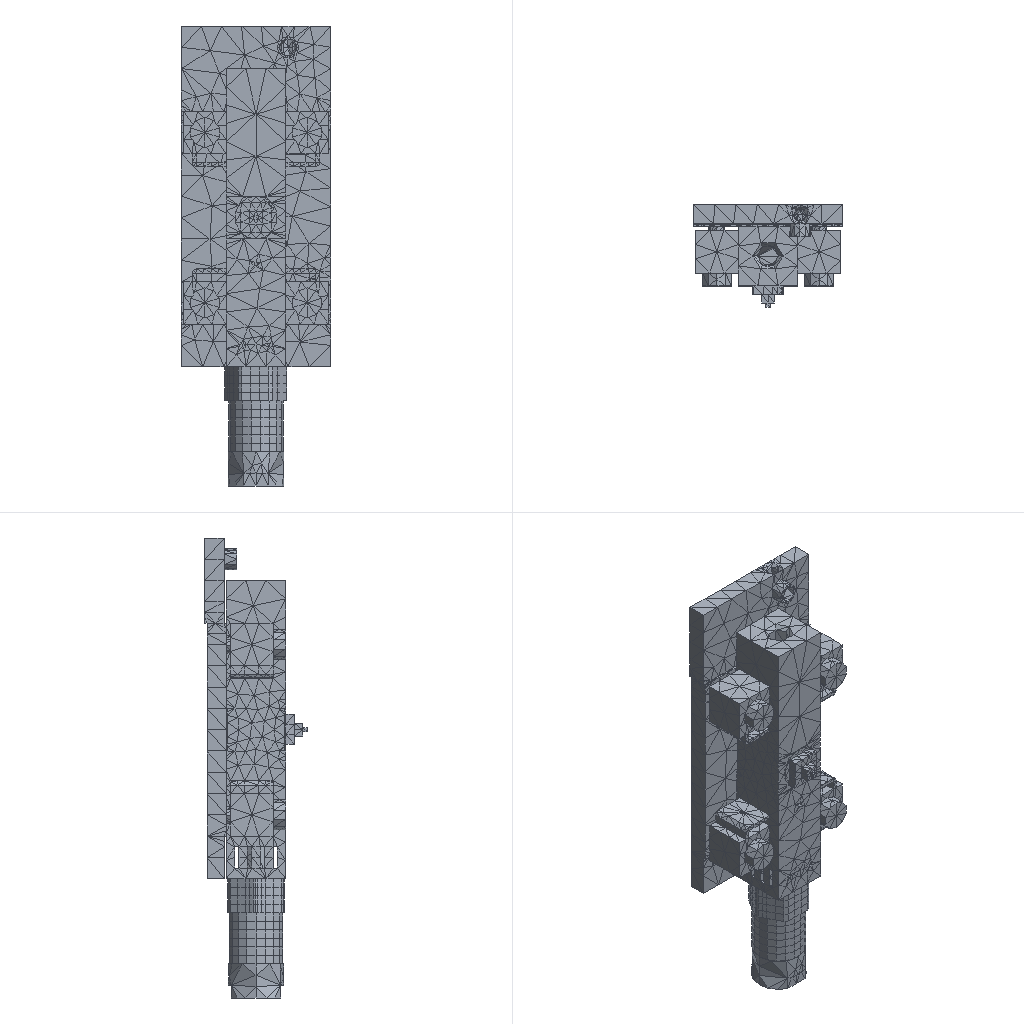Simulation study | ansys workbench
Ansys APDL input file, long lists of numbers shortened:
/batch
/config,noeldb,1     ! force off writing results to database
*get,_wallstrt,active,,time,wall
! ANSYS input file written by Workbench version 2022 R1
! File used for geometry attach: F:\ansys（分析文件汇总)\含底座模态分析\新建文件夹(4)\新建文件夹\完整版.STEP
/title,11111--____ (C5)
! ****** Begin Custom Load Command Snippet ******
/COM, ACT Extensions:
/COM,     LSDYNA, 2021.1
/COM,
! ****** End   Custom Load Command Snippet ******
*DIM,_wb_ProjectScratch_dir,string,248
_wb_ProjectScratch_dir(1) = 'F:\ansys（分析文件汇总)\含底座模态分析\_ProjectScratch\ScrD0BA\'
*DIM,_wb_SolverFiles_dir,string,248
_wb_SolverFiles_dir(1) = 'F:\ansys（分析文件汇总)\含底座模态分析\11111_files\dp0\SYS-1\MECH\'
*DIM,_wb_userfiles_dir,string,248
_wb_userfiles_dir(1) = 'F:\ansys（分析文件汇总)\含底座模态分析\11111_files\user_files\'
/com,--- Data in consistent NMM units. See Solving Units in the help system for more information.
/units,MPA
/nopr
/wb,file,start              !  signify a WB generated input file
/prep7
! Turn off shape checking because checks already performed inside WB mesher.
! See help system for more information.
SHPP,OFF,,NOWARN
/nolist
etcon,set             ! allow ANSYS to choose best KEYOP's for 180x elements, resets any applicable keyopt to MAPDL defaults
/com,*********** Nodes for the whole assembly ***********
nblock,3,,23060
(1i9,3e20.9e3)
        1    -7.593879241E+01     6.122424365E-01     1.555868903E+01
! (20963 more lines like these left out)
-1
/wb,elem,start            !  set before creation of elements
/com,*********** Elements for Body 1 "__|__-__6" ***********
et,1,187
eblock,19,solid,,4865
(19i9)
        1        1        1        1        0        0        0        0       10        0     2024     8034     8303     8491     8312    14700    15906    14703    14701
! (9729 more lines like these left out)
-1
/com,*********** Elements for Body 2 "___|__-__1" ***********
et,2,186
keyo,2,2,1          ! set full integration on SOLID186
eblock,19,solid,,35
(19i9)
        2        2        2        2        0        0        0        0       20        0      840     2544     2556     2561     2557     2579     2567     2562     2566
! (69 more lines like these left out)
-1
/com,*********** Elements for Body 3 "___|__-__1[2]" ***********
et,3,186
keyo,3,2,1          ! set full integration on SOLID186
eblock,19,solid,,35
(19i9)
        3        3        3        3        0        0        0        0       20        0      770     1924     1936     1941     1937     1959     1947     1942     1946
! (69 more lines like these left out)
-1
/com,*********** Elements for Body 4 "___|__-__1[3]" ***********
et,4,186
keyo,4,2,1          ! set full integration on SOLID186
eblock,19,solid,,35
(19i9)
        4        4        4        4        0        0        0        0       20        0      910     3164     3176     3181     3177     3199     3187     3182     3186
! (69 more lines like these left out)
-1
/com,*********** Elements for Body 5 "___|__-__1[4]" ***********
et,5,186
keyo,5,2,1          ! set full integration on SOLID186
eblock,19,solid,,35
(19i9)
        5        5        5        5        0        0        0        0       20        0      805     2234     2246     2251     2247     2269     2257     2252     2256
! (69 more lines like these left out)
-1
! (11 more sections like these left out)
/wb,elem,end               !  done creating elements
/com,*********** Send User Defined Coordinate System(s) ***********
csys,0
toffst,273.15,  ! Temperature offset from absolute zero
/com,*********** Set Reference Temperature ***********
tref,22.
/wb,mat,start              !  starting to send materials
/com,*********** Send Materials ***********
Temperature = 'TEMP' ! Temperature
TB,BISO,1,5,
TBTEMP,100
TBDATA,1,225,2091
TBTEMP,300
TBDATA,1,168,1577
TBTEMP,816
TBDATA,1,115,708
TBTEMP,1040
TBDATA,1,31,405
TBTEMP,1150
TBDATA,1,15,265
MPTEMP,,,,,,,,
MPTEMP,1,20
MPTEMP,2,100
MPTEMP,3,200
MPTEMP,4,300
MPTEMP,5,400
MPTEMP,6,500
MPTEMP,7,600
MPTEMP,8,700
MPTEMP,9,800
MPTEMP,10,900
MPTEMP,11,1000
MPTEMP,12,1100
MPTEMP,13,1200
MPDATA,EX,1, ,195000,191000,186000,180000,173000,164000,
MPDATA,EX,1, ,155000,144000,131000,117000,100000,81000,
MPDATA,EX,1, ,51000,	! tonne s^-2 mm^-1
MPTEMP,,,,,,,,
MPTEMP,,,,,,,,
MPTEMP,1,20
MPTEMP,2,100
MPTEMP,3,200
MPTEMP,4,300
MPTEMP,5,400
MPTEMP,6,500
MPTEMP,7,600
MPTEMP,8,700
MPTEMP,9,800
MPTEMP,10,900
MPTEMP,11,1000
MPTEMP,12,1100
MPTEMP,13,1200
MPDATA,NUXY,1, ,0.25,0.26,0.275,0.315,0.33,0.3,
MPDATA,NUXY,1, ,0.32,0.31,0.24,0.24,0.24,0.24,
MPDATA,NUXY,1, ,0.24,
MPTEMP,,,,,,,,
MPTEMP,,,,,,,,
MPTEMP,1,26.85
MPTEMP,2,126.85
MPTEMP,3,226.85
MPTEMP,4,326.85
MPTEMP,5,426.85
MPTEMP,6,526.85
MPTEMP,7,626.85
MPTEMP,8,726.85
MPTEMP,9,826.85
MPTEMP,10,926.85
MPTEMP,11,1026.85
MPTEMP,12,1126.85
MPTEMP,13,1226.85
MPTEMP,14,1326.85
MPTEMP,15,1426.85
MPTEMP,16,1526.85
MPTEMP,17,1626.85
MPTEMP,18,1726.85
MPTEMP,19,1826.85
MPTEMP,20,1926.85
MPTEMP,21,2026.85
MPTEMP,22,2126.85
MPTEMP,23,2226.85
MPTEMP,24,2326.85
MPTEMP,25,2426.85
MPTEMP,26,2526.85
MPTEMP,27,2626.85
MPTEMP,28,2726.85
MPDATA,DENS,1, ,7.954e-09,7.91e-09,7.864e-09,7.818e-09,7.771e-09,7.723e-09,
MPDATA,DENS,1, ,7.674e-09,7.624e-09,7.574e-09,7.523e-09,7.471e-09,7.419e-09,
! (1352 more lines like these left out)
/wb,mat,end                !  done sending materials
!************************* Model Summary ********************
!__|__-__6,	316不锈钢
,	matid,	1
!___|__-__1,	PZT-4,	matid,	2
!___|__-__1[2],	PZT-4,	matid,	3
!___|__-__1[3],	PZT-4,	matid,	4
!___|__-__1[4],	PZT-4,	matid,	5
!___|__-__1[5],	PZT-4,	matid,	6
!___|__-__1[6],	PZT-4,	matid,	7
!___|__1,	316不锈钢
,	matid,	8
!___|__1,	316不锈钢
,	matid,	9
!__|__-__5,	钨钢,	matid,	10
!__|__1,	316不锈钢
,	matid,	11
!__|__1,	316不锈钢
,	matid,	12
!__|__-__2,	316不锈钢
,	matid,	13
!__|__-__2[2],	316不锈钢
,	matid,	14
!__|__-__2[3],	316不锈钢
,	matid,	15
!__|__-__2[4],	316不锈钢
,	matid,	16
!************************* End Model Summary ********************
! get the diagonal of the bounding box. Needed later for other things
*get,_xmin,node,,mnloc,x
*get,_ymin,node,,mnloc,y
*get,_zmin,node,,mnloc,z
*get,_xmax,node,,mxloc,x
*get,_ymax,node,,mxloc,y
*get,_zmax,node,,mxloc,z
_ASMDIAG=(_xmax-_xmin)*(_xmax-_xmin)+(_ymax-_ymin)*(_ymax-_ymin)+(_zmax-_zmin)*(_zmax-_zmin)
_ASMDIAG=SQRT(_ASMDIAG)
/wb,contact,start          !  starting to send contact
/com,*********** Create Contact "接触区域" ***********
/com,            Real Constant Set For Above Contact Is 18 & 17
*set,tid,18
*set,cid,17
r,tid
r,cid
et,tid,170
et,cid,174
eblock,10,,,72
(15i9)
    15410       18       18       18        0     7091     7812     7209     7209     9306    10276     7209     9301
! (71 more lines like these left out)
-1
eblock,10,,,72
(15i9)
    15482       17       17       17        0     7091     7812     7209     7209     9306    10276     7209     9301
! (71 more lines like these left out)
-1
eblock,10,,,28
(15i9)
    15554       17       18       17        0        3        1        6        6      116      117        6      127
! (27 more lines like these left out)
-1
eblock,10,,,28
(15i9)
    15582       18       17       18        0        3        1        6        6      116      117        6      127
! (27 more lines like these left out)
-1
keyo,cid,8,2               ! auto create asymmetric contact (from Program Controlled setting)
keyo,cid,10,0              ! adjust contact stiffness each NR iteration (from Program Controlled setting)
keyo,cid,12,5              ! bonded always
keyo,cid,18,1              ! small sliding turned on by application
keyo,cid,2,0               ! augmented Lagrange (from Program Controlled setting)
keyo,cid,4,0               ! on Gauss point (from Program Controlled setting)
keyo,cid,9,1               ! ignore initial gaps/penetration
keyo,cid,7,0               ! No Prediction
rmod,tid,3,10.      ! FKN
rmod,tid,5,0.       ! ICONT
rmod,tid,6,0.       ! PINB
rmod,tid,10,0.      ! CNOF
rmod,tid,12,0.      ! FKT
rmod,tid,36,71      ! WB DSID
rmod,cid,3,10.      ! FKN
rmod,cid,5,0.       ! ICONT
rmod,cid,6,0.       ! PINB
rmod,cid,10,0.      ! CNOF
rmod,cid,12,0.      ! FKT
rmod,cid,36,71      ! WB DSID
/com,*********** Create Contact "接触区域 2" ***********
/com,            Real Constant Set For Above Contact Is 20 & 19
*set,tid,20
*set,cid,19
r,tid
r,cid
et,tid,170
et,cid,174
eblock,10,,,18
(15i9)
    15610       20       20       20        0     7098     7097     7481     7481     9356     9358     7481     9367
! (17 more lines like these left out)
-1
eblock,10,,,18
(15i9)
    15628       19       19       19        0     7098     7097     7481     7481     9356     9358     7481     9367
! (17 more lines like these left out)
-1
eblock,10,,,51
(15i9)
    15646       19       20       19        0     4333     4334     4550     4549     5009     5015     5426     5012
! (50 more lines like these left out)
-1
eblock,10,,,51
(15i9)
    15697       20       19       20        0     4333     4334     4550     4549     5009     5015     5426     5012
! (50 more lines like these left out)
-1
keyo,cid,8,2               ! auto create asymmetric contact (from Program Controlled setting)
keyo,cid,10,0              ! adjust contact stiffness each NR iteration (from Program Controlled setting)
keyo,cid,12,5              ! bonded always
keyo,cid,18,1              ! small sliding turned on by application
keyo,cid,2,0               ! augmented Lagrange (from Program Controlled setting)
keyo,cid,4,0               ! on Gauss point (from Program Controlled setting)
keyo,cid,9,1               ! ignore initial gaps/penetration
keyo,cid,7,0               ! No Prediction
rmod,tid,3,10.      ! FKN
rmod,tid,5,0.       ! ICONT
rmod,tid,6,0.       ! PINB
rmod,tid,10,0.      ! CNOF
rmod,tid,12,0.      ! FKT
rmod,tid,36,74      ! WB DSID
rmod,cid,3,10.      ! FKN
rmod,cid,5,0.       ! ICONT
rmod,cid,6,0.       ! PINB
rmod,cid,10,0.      ! CNOF
rmod,cid,12,0.      ! FKT
rmod,cid,36,74      ! WB DSID
/com,*********** Create Contact "接触区域 3" ***********
/com,            Real Constant Set For Above Contact Is 22 & 21
*set,tid,22
*set,cid,21
r,tid
r,cid
et,tid,170
et,cid,174
eblock,10,,,66
(15i9)
    15748       22       22       22        0     7771     7979     7048     7048    13698     8980     7048     8977
! (65 more lines like these left out)
-1
eblock,10,,,66
(15i9)
    15814       21       21       21        0     7771     7979     7048     7048    13698     8980     7048     8977
! (65 more lines like these left out)
-1
eblock,10,,,127
(15i9)
    15880       21       22       21        0     5467     5468     5596     5596     5886     5896     5596     5889
! (126 more lines like these left out)
-1
eblock,10,,,127
(15i9)
    16007       22       21       22        0     5467     5468     5596     5596     5886     5896     5596     5889
! (126 more lines like these left out)
-1
keyo,cid,8,2               ! auto create asymmetric contact (from Program Controlled setting)
keyo,cid,10,0              ! adjust contact stiffness each NR iteration (from Program Controlled setting)
keyo,cid,12,5              ! bonded always
keyo,cid,18,1              ! small sliding turned on by application
keyo,cid,2,0               ! augmented Lagrange (from Program Controlled setting)
keyo,cid,4,0               ! on Gauss point (from Program Controlled setting)
keyo,cid,9,1               ! ignore initial gaps/penetration
keyo,cid,7,0               ! No Prediction
rmod,tid,3,10.      ! FKN
rmod,tid,5,0.       ! ICONT
rmod,tid,6,0.       ! PINB
rmod,tid,10,0.      ! CNOF
rmod,tid,12,0.      ! FKT
rmod,tid,36,77      ! WB DSID
rmod,cid,3,10.      ! FKN
rmod,cid,5,0.       ! ICONT
rmod,cid,6,0.       ! PINB
rmod,cid,10,0.      ! CNOF
rmod,cid,12,0.      ! FKT
rmod,cid,36,77      ! WB DSID
/com,*********** Create Contact "接触区域 4" ***********
/com,            Real Constant Set For Above Contact Is 24 & 23
*set,tid,24
*set,cid,23
r,tid
r,cid
et,tid,170
et,cid,174
eblock,10,,,24
(15i9)
    16134       24       24       24        0     7044     7881     7498     7498     8932    12249     7498     8929
! (23 more lines like these left out)
-1
eblock,10,,,24
(15i9)
    16158       23       23       23        0     7044     7881     7498     7498     8932    12249     7498     8929
! (23 more lines like these left out)
-1
eblock,10,,,36
(15i9)
    16182       23       24       23        0     3540     3541     3569     3569     3910     3915     3569     3912
! (35 more lines like these left out)
-1
eblock,10,,,36
(15i9)
    16218       24       23       24        0     3540     3541     3569     3569     3910     3915     3569     3912
! (35 more lines like these left out)
-1
keyo,cid,8,2               ! auto create asymmetric contact (from Program Controlled setting)
keyo,cid,10,0              ! adjust contact stiffness each NR iteration (from Program Controlled setting)
keyo,cid,12,5              ! bonded always
keyo,cid,18,1              ! small sliding turned on by application
keyo,cid,2,0               ! augmented Lagrange (from Program Controlled setting)
keyo,cid,4,0               ! on Gauss point (from Program Controlled setting)
keyo,cid,9,1               ! ignore initial gaps/penetration
keyo,cid,7,0               ! No Prediction
rmod,tid,3,10.      ! FKN
rmod,tid,5,0.       ! ICONT
rmod,tid,6,0.       ! PINB
rmod,tid,10,0.      ! CNOF
rmod,tid,12,0.      ! FKT
rmod,tid,36,80      ! WB DSID
rmod,cid,3,10.      ! FKN
rmod,cid,5,0.       ! ICONT
rmod,cid,6,0.       ! PINB
rmod,cid,10,0.      ! CNOF
rmod,cid,12,0.      ! FKT
rmod,cid,36,80      ! WB DSID
/com,*********** Create Contact "接触区域 5" ***********
/com,            Real Constant Set For Above Contact Is 26 & 25
*set,tid,26
*set,cid,25
r,tid
r,cid
et,tid,170
et,cid,174
eblock,10,,,200
(15i9)
    16254       26       26       26        0     8149     8178     8152     8152    15277    15300     8152    15274
! (199 more lines like these left out)
-1
eblock,10,,,200
(15i9)
    16454       25       25       25        0     8149     8178     8152     8152    15277    15300     8152    15274
! (199 more lines like these left out)
-1
eblock,10,,,158
(15i9)
    16654       25       26       25        0    16812    16862    16828    16828    20339    20448    16828    20337
! (157 more lines like these left out)
-1
eblock,10,,,158
(15i9)
    16812       26       25       26        0    16812    16862    16828    16828    20339    20448    16828    20337
! (157 more lines like these left out)
-1
keyo,cid,8,2               ! auto create asymmetric contact (from Program Controlled setting)
keyo,cid,10,0              ! adjust contact stiffness each NR iteration (from Program Controlled setting)
keyo,cid,12,5              ! bonded always
keyo,cid,18,1              ! small sliding turned on by application
keyo,cid,2,0               ! augmented Lagrange (from Program Controlled setting)
keyo,cid,4,0               ! on Gauss point (from Program Controlled setting)
keyo,cid,9,1               ! ignore initial gaps/penetration
keyo,cid,7,0               ! No Prediction
rmod,tid,3,10.      ! FKN
rmod,tid,5,0.       ! ICONT
rmod,tid,6,0.       ! PINB
rmod,tid,10,0.      ! CNOF
rmod,tid,12,0.      ! FKT
rmod,tid,36,83      ! WB DSID
rmod,cid,3,10.      ! FKN
rmod,cid,5,0.       ! ICONT
rmod,cid,6,0.       ! PINB
rmod,cid,10,0.      ! CNOF
rmod,cid,12,0.      ! FKT
rmod,cid,36,83      ! WB DSID
! (18 more sections like these left out)
/wb,contact,end            !  done creating contacts
/golist
/wb,load,start             !  starting to send loads
/com,*********** Define Force Using Surface Effect Elements ***********
local,12,0,0.,0.,0.,0.,0.,0.
csys,0
et,63,154
eblock,10,,,260
(15i9)
    19468       63       63       63       12    16254    16574    16912    16912    17146    19278    16912    17149
! (259 more lines like these left out)
-1
esel,s,type,,63
keyop,63,2,1                ! Apply load in local coordinate system
keyop,63,7,1                ! Use original area so load is constant in large deformation
esel,all
*DIM,_loadvari160x,TABLE,1,1,1,TIME
! Time values
*TAXIS,_loadvari160x(1),1,1.
! Load values
_loadvari160x(1,1,1) = 0.
*DIM,_loadvari160xi,TABLE,1,1,1,TIME
! Time values
*TAXIS,_loadvari160xi(1),1,1.
! Load values
_loadvari160xi(1,1,1) = 0.
*DIM,_loadvari160y,TABLE,1,1,1,TIME
! Time values
*TAXIS,_loadvari160y(1),1,1.
! Load values
_loadvari160y(1,1,1) = -0.1864
*DIM,_loadvari160yi,TABLE,1,1,1,TIME
! Time values
*TAXIS,_loadvari160yi(1),1,1.
! Load values
_loadvari160yi(1,1,1) = 0.
*DIM,_loadvari160z,TABLE,1,1,1,TIME
! Time values
*TAXIS,_loadvari160z(1),1,1.
! Load values
_loadvari160z(1,1,1) = 0.
*DIM,_loadvari160zi,TABLE,1,1,1,TIME
! Time values
*TAXIS,_loadvari160zi(1),1,1.
! Load values
_loadvari160zi(1,1,1) = 0.
/gst,on,on
fini
*get,_numnode,node,0,count
*get,_numelem,elem,0,count
*get, _MAXELEMNUM, elem, 0, NUM, MAX
*get, _MAXNODENUM, node, 0, NUM, MAX
*get, _MAXELEMTYPE, etyp, 0, NUM, MAX
*get, _MAXREALCONST, real, 0, NUM, MAX
/go
/wb,load,end               !  done creating loads
/com,--- Number of total nodes = %_numnode%
/com,--- Number of contact elements = 4318
/com,--- Number of spring elements = 0
/com,--- Number of bearing elements = 0
/com,--- Number of solid elements = 9315
/com,--- Number of condensed parts = 0
/com,--- Number of total elements = %_numelem%
*get,_wallbsol,active,,time,wall
/com,*********** Performing Modal Solve ***********
/solu
antype,2
modcontrol,on
thexpand,off     ! ignore thermal strains
mxpand,,,,yes,,no     ! expand element results for stress/strains, but not write them to file.mode
outres,erase
outres,all,none
outres,nsol,all
outres,eangl,all
outres,etmp,all
outres,veng,all
outres,strs,all
outres,epel,all
outres,rsol,all
outres,cont,all
modopt,lanb,200,25000.,140000.
fdele,all,all
sfdele,all,all
sfedele,all,all,all
acel,0,0,0                 ! zero out the acceleration
/com,*********** Setting and Solving Each Load Step ***********
esel,s,type,,63
nsle
sfe,all,2,pres,1,1
nsel,all
esel,all
solve
/com,**********************
/com *************** Write FE CONNECTORS *********
CEWRITE,file,ce,,INTE
fini
*get,_wallasol,active,,time,wall
/com,*********** Performing MSUP Harmonic Solve ***********
/solu
antype,harm
hropt,msup
thexpand,off     ! ignore thermal strains
hrout,off
kbc,1
harfrq,50000.,70000.
nsub,80
fdele,all,all
sfdele,all,all
sfedele,all,all,all
acel,0,0,0                 ! zero out the acceleration
lvscale,0,1
/com,*********** Scaling Each Load Step for MSUP Solve ***********
lvscale,%_loadvari160y%,1
! *********** WB SOLVE COMMAND ***********
! check interactive state
*get,ANSINTER_,active,,int
*if,ANSINTER_,ne,0,then
/eof
*endif
solve
fini
*get,_wallasol,active,,time,wall
! ------- MSUP EXPANSION PASS -------
/solu
expass,on
hrexp,all
outres,erase
outres,all,none
outres,nsol,all
outres,eangl,all
outres,etmp,all
outres,veng,all
outres,strs,all
outres,epel,all
outres,rsol,all
outres,cont,all
numexp,all,,,yes        ! expand results at all freq. and calculate requested result items
! *********** WB SOLVE COMMAND ***********
! check interactive state
*get,ANSINTER_,active,,int
*if,ANSINTER_,ne,0,then
/eof
*endif
solve
/com *************** Write FE CONNECTORS *********
CEWRITE,file,ce,,INTE
fini
/post1
xmlo,ENCODING,ISO-8859-1
xmlo,parm
/xml,parm,xml
fini
/gopr
*get,_walldone,active,,time,wall
_preptime=(_wallbsol-_wallstrt)*3600
_solvtime=(_wallasol-_wallbsol)*3600
_posttime=(_walldone-_wallasol)*3600
_totaltim=(_walldone-_wallstrt)*3600
*get,_dlbratio,active,0,solu,dlbr
*get,_combtime,active,0,solu,comb
*get,_ssmode,active,0,solu,ssmm
*get,_ndofs,active,0,solu,ndof
/fclean				!clean distributed files
/com,--- Total number of nodes = %_numnode%
/com,--- Total number of elements = %_numelem%
/com,--- Element load balance ratio = %_dlbratio%
/com,--- Time to combine distributed files = %_combtime%
/com,--- Sparse memory mode = %_ssmode%
/com,--- Number of DOF = %_ndofs%
/wb,file,end               ! done with WB generated input